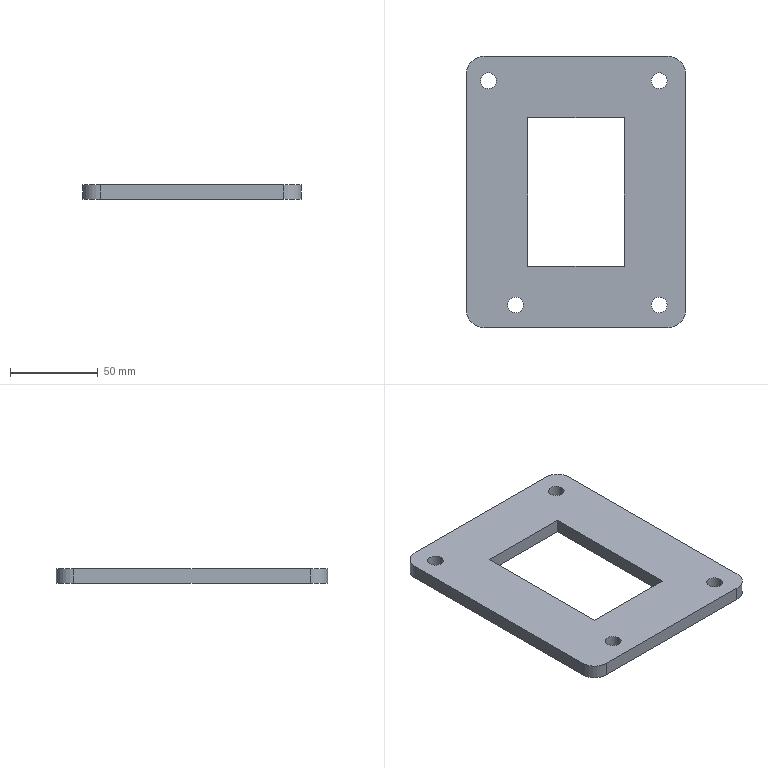Part | SolidWorks | features FlatPattern 1, SMBaseFlange 1, SheetMetal 1 | 1 solid | 22 faces | box 125 x 155 x 8 mm | volume 114878 mm3 | cylinder 12 | plane 10 | commonest cylinder face diameters 9 x8 20 x4
STEP:
#1=CARTESIAN_POINT('',(-51.5,13.,8.));
#2=VERTEX_POINT('',#1);
#3=CARTESIAN_POINT('',(-42.5,13.,8.));
#4=VERTEX_POINT('',#3);
#5=CARTESIAN_POINT('',(-47.,13.,8.));
#6=DIRECTION('',(0.,0.,1.));
#7=DIRECTION('',(1.,0.,0.));
#8=AXIS2_PLACEMENT_3D('',#5,#6,#7);
#9=CIRCLE('',#8,4.5);
#10=EDGE_CURVE('',#2,#4,#9,.T.);
#11=ORIENTED_EDGE('',*,*,#10,.T.);
#12=CARTESIAN_POINT('',(-42.5,13.,0.));
#13=VERTEX_POINT('',#12);
#14=CARTESIAN_POINT('',(-42.5,13.,8.));
#15=DIRECTION('',(0.,0.,-1.));
#16=VECTOR('',#15,1000.);
#17=LINE('',#14,#16);
#18=EDGE_CURVE('',#4,#13,#17,.T.);
#19=ORIENTED_EDGE('',*,*,#18,.T.);
#20=CARTESIAN_POINT('',(-51.5,13.,0.));
#21=VERTEX_POINT('',#20);
#22=CARTESIAN_POINT('',(-47.,13.,0.));
#23=DIRECTION('',(0.,0.,1.));
#24=DIRECTION('',(1.,0.,0.));
#25=AXIS2_PLACEMENT_3D('',#22,#23,#24);
#26=CIRCLE('',#25,4.5);
#27=EDGE_CURVE('',#21,#13,#26,.T.);
#28=ORIENTED_EDGE('',*,*,#27,.F.);
#29=CARTESIAN_POINT('',(-51.5,13.,8.));
#30=DIRECTION('',(0.,0.,-1.));
#31=VECTOR('',#30,1000.);
#32=LINE('',#29,#31);
#33=EDGE_CURVE('',#2,#21,#32,.T.);
#34=ORIENTED_EDGE('',*,*,#33,.F.);
#35=EDGE_LOOP('',(#11,#19,#28,#34));
#36=FACE_OUTER_BOUND('',#35,.T.);
#37=CARTESIAN_POINT('',(-47.,13.,8.));
#38=DIRECTION('',(0.,0.,-1.));
#39=DIRECTION('',(-1.,0.,0.));
#40=AXIS2_PLACEMENT_3D('',#37,#38,#39);
#41=CYLINDRICAL_SURFACE('',#40,4.5);
#42=ADVANCED_FACE('',(#36),#41,.F.);
#43=CARTESIAN_POINT('',(30.5,13.,8.));
#44=VERTEX_POINT('',#43);
#45=CARTESIAN_POINT('',(39.5,13.,8.));
#46=VERTEX_POINT('',#45);
#47=CARTESIAN_POINT('',(35.,13.,8.));
#48=DIRECTION('',(0.,0.,1.));
#49=DIRECTION('',(1.,0.,0.));
#50=AXIS2_PLACEMENT_3D('',#47,#48,#49);
#51=CIRCLE('',#50,4.5);
#52=EDGE_CURVE('',#44,#46,#51,.T.);
#53=ORIENTED_EDGE('',*,*,#52,.T.);
#54=CARTESIAN_POINT('',(39.5,13.,0.));
#55=VERTEX_POINT('',#54);
#56=CARTESIAN_POINT('',(39.5,13.,8.));
#57=DIRECTION('',(0.,0.,-1.));
#58=VECTOR('',#57,1000.);
#59=LINE('',#56,#58);
#60=EDGE_CURVE('',#46,#55,#59,.T.);
#61=ORIENTED_EDGE('',*,*,#60,.T.);
#62=CARTESIAN_POINT('',(30.5,13.,0.));
#63=VERTEX_POINT('',#62);
#64=CARTESIAN_POINT('',(35.,13.,0.));
#65=DIRECTION('',(0.,0.,1.));
#66=DIRECTION('',(1.,0.,0.));
#67=AXIS2_PLACEMENT_3D('',#64,#65,#66);
#68=CIRCLE('',#67,4.5);
#69=EDGE_CURVE('',#63,#55,#68,.T.);
#70=ORIENTED_EDGE('',*,*,#69,.F.);
#71=CARTESIAN_POINT('',(30.5,13.,8.));
#72=DIRECTION('',(0.,0.,-1.));
#73=VECTOR('',#72,1000.);
#74=LINE('',#71,#73);
#75=EDGE_CURVE('',#44,#63,#74,.T.);
#76=ORIENTED_EDGE('',*,*,#75,.F.);
#77=EDGE_LOOP('',(#53,#61,#70,#76));
#78=FACE_OUTER_BOUND('',#77,.T.);
#79=CARTESIAN_POINT('',(35.,13.,8.));
#80=DIRECTION('',(0.,0.,-1.));
#81=DIRECTION('',(-1.,0.,0.));
#82=AXIS2_PLACEMENT_3D('',#79,#80,#81);
#83=CYLINDRICAL_SURFACE('',#82,4.5);
#84=ADVANCED_FACE('',(#78),#83,.F.);
#85=CARTESIAN_POINT('',(30.5,141.,8.));
#86=VERTEX_POINT('',#85);
#87=CARTESIAN_POINT('',(39.5,141.,8.));
#88=VERTEX_POINT('',#87);
#89=CARTESIAN_POINT('',(35.,141.,8.));
#90=DIRECTION('',(0.,0.,1.));
#91=DIRECTION('',(1.,0.,0.));
#92=AXIS2_PLACEMENT_3D('',#89,#90,#91);
#93=CIRCLE('',#92,4.5);
#94=EDGE_CURVE('',#86,#88,#93,.T.);
#95=ORIENTED_EDGE('',*,*,#94,.T.);
#96=CARTESIAN_POINT('',(39.5,141.,0.));
#97=VERTEX_POINT('',#96);
#98=CARTESIAN_POINT('',(39.5,141.,8.));
#99=DIRECTION('',(0.,0.,-1.));
#100=VECTOR('',#99,1000.);
#101=LINE('',#98,#100);
#102=EDGE_CURVE('',#88,#97,#101,.T.);
#103=ORIENTED_EDGE('',*,*,#102,.T.);
#104=CARTESIAN_POINT('',(30.5,141.,0.));
#105=VERTEX_POINT('',#104);
#106=CARTESIAN_POINT('',(35.,141.,0.));
#107=DIRECTION('',(0.,0.,1.));
#108=DIRECTION('',(1.,0.,0.));
#109=AXIS2_PLACEMENT_3D('',#106,#107,#108);
#110=CIRCLE('',#109,4.5);
#111=EDGE_CURVE('',#105,#97,#110,.T.);
#112=ORIENTED_EDGE('',*,*,#111,.F.);
#113=CARTESIAN_POINT('',(30.5,141.,8.));
#114=DIRECTION('',(0.,0.,-1.));
#115=VECTOR('',#114,1000.);
#116=LINE('',#113,#115);
#117=EDGE_CURVE('',#86,#105,#116,.T.);
#118=ORIENTED_EDGE('',*,*,#117,.F.);
#119=EDGE_LOOP('',(#95,#103,#112,#118));
#120=FACE_OUTER_BOUND('',#119,.T.);
#121=CARTESIAN_POINT('',(35.,141.,8.));
#122=DIRECTION('',(0.,0.,-1.));
#123=DIRECTION('',(-1.,0.,0.));
#124=AXIS2_PLACEMENT_3D('',#121,#122,#123);
#125=CYLINDRICAL_SURFACE('',#124,4.5);
#126=ADVANCED_FACE('',(#120),#125,.F.);
#127=CARTESIAN_POINT('',(-67.,141.,8.));
#128=VERTEX_POINT('',#127);
#129=CARTESIAN_POINT('',(-58.,141.,8.));
#130=VERTEX_POINT('',#129);
#131=CARTESIAN_POINT('',(-62.5,141.,8.));
#132=DIRECTION('',(0.,0.,1.));
#133=DIRECTION('',(1.,0.,0.));
#134=AXIS2_PLACEMENT_3D('',#131,#132,#133);
#135=CIRCLE('',#134,4.5);
#136=EDGE_CURVE('',#128,#130,#135,.T.);
#137=ORIENTED_EDGE('',*,*,#136,.T.);
#138=CARTESIAN_POINT('',(-58.,141.,0.));
#139=VERTEX_POINT('',#138);
#140=CARTESIAN_POINT('',(-58.,141.,8.));
#141=DIRECTION('',(0.,0.,-1.));
#142=VECTOR('',#141,1000.);
#143=LINE('',#140,#142);
#144=EDGE_CURVE('',#130,#139,#143,.T.);
#145=ORIENTED_EDGE('',*,*,#144,.T.);
#146=CARTESIAN_POINT('',(-67.,141.,0.));
#147=VERTEX_POINT('',#146);
#148=CARTESIAN_POINT('',(-62.5,141.,0.));
#149=DIRECTION('',(0.,0.,1.));
#150=DIRECTION('',(1.,0.,0.));
#151=AXIS2_PLACEMENT_3D('',#148,#149,#150);
#152=CIRCLE('',#151,4.5);
#153=EDGE_CURVE('',#147,#139,#152,.T.);
#154=ORIENTED_EDGE('',*,*,#153,.F.);
#155=CARTESIAN_POINT('',(-67.,141.,8.));
#156=DIRECTION('',(0.,0.,-1.));
#157=VECTOR('',#156,1000.);
#158=LINE('',#155,#157);
#159=EDGE_CURVE('',#128,#147,#158,.T.);
#160=ORIENTED_EDGE('',*,*,#159,.F.);
#161=EDGE_LOOP('',(#137,#145,#154,#160));
#162=FACE_OUTER_BOUND('',#161,.T.);
#163=CARTESIAN_POINT('',(-62.5,141.,8.));
#164=DIRECTION('',(0.,0.,-1.));
#165=DIRECTION('',(-1.,0.,0.));
#166=AXIS2_PLACEMENT_3D('',#163,#164,#165);
#167=CYLINDRICAL_SURFACE('',#166,4.5);
#168=ADVANCED_FACE('',(#162),#167,.F.);
#169=CARTESIAN_POINT('',(40.,0.,8.));
#170=VERTEX_POINT('',#169);
#171=CARTESIAN_POINT('',(50.,10.,8.));
#172=VERTEX_POINT('',#171);
#173=CARTESIAN_POINT('',(40.,10.,8.));
#174=DIRECTION('',(0.,0.,1.));
#175=DIRECTION('',(-1.,0.,0.));
#176=AXIS2_PLACEMENT_3D('',#173,#174,#175);
#177=CIRCLE('',#176,10.);
#178=EDGE_CURVE('',#170,#172,#177,.T.);
#179=ORIENTED_EDGE('',*,*,#178,.T.);
#180=CARTESIAN_POINT('',(50.,145.,8.));
#181=VERTEX_POINT('',#180);
#182=CARTESIAN_POINT('',(50.,145.,8.));
#183=DIRECTION('',(0.,1.,0.));
#184=VECTOR('',#183,1000.);
#185=LINE('',#182,#184);
#186=EDGE_CURVE('',#172,#181,#185,.T.);
#187=ORIENTED_EDGE('',*,*,#186,.T.);
#188=CARTESIAN_POINT('',(40.,155.,8.));
#189=VERTEX_POINT('',#188);
#190=CARTESIAN_POINT('',(40.,145.,8.));
#191=DIRECTION('',(0.,0.,1.));
#192=DIRECTION('',(-1.,0.,0.));
#193=AXIS2_PLACEMENT_3D('',#190,#191,#192);
#194=CIRCLE('',#193,10.);
#195=EDGE_CURVE('',#181,#189,#194,.T.);
#196=ORIENTED_EDGE('',*,*,#195,.T.);
#197=CARTESIAN_POINT('',(-65.,155.,8.));
#198=VERTEX_POINT('',#197);
#199=CARTESIAN_POINT('',(40.,155.,8.));
#200=DIRECTION('',(-1.,0.,0.));
#201=VECTOR('',#200,1000.);
#202=LINE('',#199,#201);
#203=EDGE_CURVE('',#189,#198,#202,.T.);
#204=ORIENTED_EDGE('',*,*,#203,.T.);
#205=CARTESIAN_POINT('',(-75.,145.,8.));
#206=VERTEX_POINT('',#205);
#207=CARTESIAN_POINT('',(-65.,145.,8.));
#208=DIRECTION('',(0.,0.,1.));
#209=DIRECTION('',(1.,0.,0.));
#210=AXIS2_PLACEMENT_3D('',#207,#208,#209);
#211=CIRCLE('',#210,10.);
#212=EDGE_CURVE('',#198,#206,#211,.T.);
#213=ORIENTED_EDGE('',*,*,#212,.T.);
#214=CARTESIAN_POINT('',(-75.,10.,8.));
#215=VERTEX_POINT('',#214);
#216=CARTESIAN_POINT('',(-75.,145.,8.));
#217=DIRECTION('',(0.,-1.,0.));
#218=VECTOR('',#217,1000.);
#219=LINE('',#216,#218);
#220=EDGE_CURVE('',#206,#215,#219,.T.);
#221=ORIENTED_EDGE('',*,*,#220,.T.);
#222=CARTESIAN_POINT('',(-65.,0.,8.));
#223=VERTEX_POINT('',#222);
#224=CARTESIAN_POINT('',(-65.,10.,8.));
#225=DIRECTION('',(0.,0.,1.));
#226=DIRECTION('',(-1.,0.,0.));
#227=AXIS2_PLACEMENT_3D('',#224,#225,#226);
#228=CIRCLE('',#227,10.);
#229=EDGE_CURVE('',#215,#223,#228,.T.);
#230=ORIENTED_EDGE('',*,*,#229,.T.);
#231=CARTESIAN_POINT('',(40.,0.,8.));
#232=DIRECTION('',(1.,0.,0.));
#233=VECTOR('',#232,1000.);
#234=LINE('',#231,#233);
#235=EDGE_CURVE('',#223,#170,#234,.T.);
#236=ORIENTED_EDGE('',*,*,#235,.T.);
#237=EDGE_LOOP('',(#179,#187,#196,#204,#213,#221,#230,#236));
#238=FACE_OUTER_BOUND('',#237,.T.);
#239=CARTESIAN_POINT('',(15.,35.,8.));
#240=VERTEX_POINT('',#239);
#241=CARTESIAN_POINT('',(15.,120.,8.));
#242=VERTEX_POINT('',#241);
#243=CARTESIAN_POINT('',(15.,120.,8.));
#244=DIRECTION('',(0.,1.,0.));
#245=VECTOR('',#244,1000.);
#246=LINE('',#243,#245);
#247=EDGE_CURVE('',#240,#242,#246,.T.);
#248=ORIENTED_EDGE('',*,*,#247,.F.);
#249=CARTESIAN_POINT('',(-40.,35.,8.));
#250=VERTEX_POINT('',#249);
#251=CARTESIAN_POINT('',(15.,35.,8.));
#252=DIRECTION('',(1.,0.,0.));
#253=VECTOR('',#252,1000.);
#254=LINE('',#251,#253);
#255=EDGE_CURVE('',#250,#240,#254,.T.);
#256=ORIENTED_EDGE('',*,*,#255,.F.);
#257=CARTESIAN_POINT('',(-40.,120.,8.));
#258=VERTEX_POINT('',#257);
#259=CARTESIAN_POINT('',(-40.,120.,8.));
#260=DIRECTION('',(0.,-1.,0.));
#261=VECTOR('',#260,1000.);
#262=LINE('',#259,#261);
#263=EDGE_CURVE('',#258,#250,#262,.T.);
#264=ORIENTED_EDGE('',*,*,#263,.F.);
#265=CARTESIAN_POINT('',(15.,120.,8.));
#266=DIRECTION('',(-1.,0.,0.));
#267=VECTOR('',#266,1000.);
#268=LINE('',#265,#267);
#269=EDGE_CURVE('',#242,#258,#268,.T.);
#270=ORIENTED_EDGE('',*,*,#269,.F.);
#271=EDGE_LOOP('',(#248,#256,#264,#270));
#272=FACE_BOUND('',#271,.T.);
#273=ORIENTED_EDGE('',*,*,#136,.F.);
#274=CARTESIAN_POINT('',(-62.5,141.,8.));
#275=DIRECTION('',(0.,0.,1.));
#276=DIRECTION('',(1.,0.,0.));
#277=AXIS2_PLACEMENT_3D('',#274,#275,#276);
#278=CIRCLE('',#277,4.5);
#279=EDGE_CURVE('',#130,#128,#278,.T.);
#280=ORIENTED_EDGE('',*,*,#279,.F.);
#281=EDGE_LOOP('',(#273,#280));
#282=FACE_BOUND('',#281,.T.);
#283=ORIENTED_EDGE('',*,*,#94,.F.);
#284=CARTESIAN_POINT('',(35.,141.,8.));
#285=DIRECTION('',(0.,0.,1.));
#286=DIRECTION('',(1.,0.,0.));
#287=AXIS2_PLACEMENT_3D('',#284,#285,#286);
#288=CIRCLE('',#287,4.5);
#289=EDGE_CURVE('',#88,#86,#288,.T.);
#290=ORIENTED_EDGE('',*,*,#289,.F.);
#291=EDGE_LOOP('',(#283,#290));
#292=FACE_BOUND('',#291,.T.);
#293=ORIENTED_EDGE('',*,*,#52,.F.);
#294=CARTESIAN_POINT('',(35.,13.,8.));
#295=DIRECTION('',(0.,0.,1.));
#296=DIRECTION('',(1.,0.,0.));
#297=AXIS2_PLACEMENT_3D('',#294,#295,#296);
#298=CIRCLE('',#297,4.5);
#299=EDGE_CURVE('',#46,#44,#298,.T.);
#300=ORIENTED_EDGE('',*,*,#299,.F.);
#301=EDGE_LOOP('',(#293,#300));
#302=FACE_BOUND('',#301,.T.);
#303=ORIENTED_EDGE('',*,*,#10,.F.);
#304=CARTESIAN_POINT('',(-47.,13.,8.));
#305=DIRECTION('',(0.,0.,1.));
#306=DIRECTION('',(1.,0.,0.));
#307=AXIS2_PLACEMENT_3D('',#304,#305,#306);
#308=CIRCLE('',#307,4.5);
#309=EDGE_CURVE('',#4,#2,#308,.T.);
#310=ORIENTED_EDGE('',*,*,#309,.F.);
#311=EDGE_LOOP('',(#303,#310));
#312=FACE_BOUND('',#311,.T.);
#313=CARTESIAN_POINT('',(40.,10.,8.));
#314=DIRECTION('',(0.,0.,-1.));
#315=DIRECTION('',(-1.,0.,0.));
#316=AXIS2_PLACEMENT_3D('',#313,#314,#315);
#317=PLANE('',#316);
#318=ADVANCED_FACE('',(#238,#272,#282,#292,#302,#312),#317,.F.);
#319=ORIENTED_EDGE('',*,*,#69,.T.);
#320=CARTESIAN_POINT('',(35.,13.,0.));
#321=DIRECTION('',(0.,0.,1.));
#322=DIRECTION('',(1.,0.,0.));
#323=AXIS2_PLACEMENT_3D('',#320,#321,#322);
#324=CIRCLE('',#323,4.5);
#325=EDGE_CURVE('',#55,#63,#324,.T.);
#326=ORIENTED_EDGE('',*,*,#325,.T.);
#327=EDGE_LOOP('',(#319,#326));
#328=FACE_BOUND('',#327,.T.);
#329=ORIENTED_EDGE('',*,*,#153,.T.);
#330=CARTESIAN_POINT('',(-62.5,141.,0.));
#331=DIRECTION('',(0.,0.,1.));
#332=DIRECTION('',(1.,0.,0.));
#333=AXIS2_PLACEMENT_3D('',#330,#331,#332);
#334=CIRCLE('',#333,4.5);
#335=EDGE_CURVE('',#139,#147,#334,.T.);
#336=ORIENTED_EDGE('',*,*,#335,.T.);
#337=EDGE_LOOP('',(#329,#336));
#338=FACE_BOUND('',#337,.T.);
#339=CARTESIAN_POINT('',(40.,0.,0.));
#340=VERTEX_POINT('',#339);
#341=CARTESIAN_POINT('',(50.,10.,0.));
#342=VERTEX_POINT('',#341);
#343=CARTESIAN_POINT('',(40.,10.,0.));
#344=DIRECTION('',(0.,0.,1.));
#345=DIRECTION('',(-1.,0.,0.));
#346=AXIS2_PLACEMENT_3D('',#343,#344,#345);
#347=CIRCLE('',#346,10.);
#348=EDGE_CURVE('',#340,#342,#347,.T.);
#349=ORIENTED_EDGE('',*,*,#348,.F.);
#350=CARTESIAN_POINT('',(-65.,0.,0.));
#351=VERTEX_POINT('',#350);
#352=CARTESIAN_POINT('',(40.,0.,0.));
#353=DIRECTION('',(1.,0.,0.));
#354=VECTOR('',#353,1000.);
#355=LINE('',#352,#354);
#356=EDGE_CURVE('',#351,#340,#355,.T.);
#357=ORIENTED_EDGE('',*,*,#356,.F.);
#358=CARTESIAN_POINT('',(-75.,10.,0.));
#359=VERTEX_POINT('',#358);
#360=CARTESIAN_POINT('',(-65.,10.,0.));
#361=DIRECTION('',(0.,0.,1.));
#362=DIRECTION('',(-1.,0.,0.));
#363=AXIS2_PLACEMENT_3D('',#360,#361,#362);
#364=CIRCLE('',#363,10.);
#365=EDGE_CURVE('',#359,#351,#364,.T.);
#366=ORIENTED_EDGE('',*,*,#365,.F.);
#367=CARTESIAN_POINT('',(-75.,145.,0.));
#368=VERTEX_POINT('',#367);
#369=CARTESIAN_POINT('',(-75.,145.,0.));
#370=DIRECTION('',(0.,-1.,0.));
#371=VECTOR('',#370,1000.);
#372=LINE('',#369,#371);
#373=EDGE_CURVE('',#368,#359,#372,.T.);
#374=ORIENTED_EDGE('',*,*,#373,.F.);
#375=CARTESIAN_POINT('',(-65.,155.,0.));
#376=VERTEX_POINT('',#375);
#377=CARTESIAN_POINT('',(-65.,145.,0.));
#378=DIRECTION('',(0.,0.,1.));
#379=DIRECTION('',(1.,0.,0.));
#380=AXIS2_PLACEMENT_3D('',#377,#378,#379);
#381=CIRCLE('',#380,10.);
#382=EDGE_CURVE('',#376,#368,#381,.T.);
#383=ORIENTED_EDGE('',*,*,#382,.F.);
#384=CARTESIAN_POINT('',(40.,155.,0.));
#385=VERTEX_POINT('',#384);
#386=CARTESIAN_POINT('',(40.,155.,0.));
#387=DIRECTION('',(-1.,0.,0.));
#388=VECTOR('',#387,1000.);
#389=LINE('',#386,#388);
#390=EDGE_CURVE('',#385,#376,#389,.T.);
#391=ORIENTED_EDGE('',*,*,#390,.F.);
#392=CARTESIAN_POINT('',(50.,145.,0.));
#393=VERTEX_POINT('',#392);
#394=CARTESIAN_POINT('',(40.,145.,0.));
#395=DIRECTION('',(0.,0.,1.));
#396=DIRECTION('',(-1.,0.,0.));
#397=AXIS2_PLACEMENT_3D('',#394,#395,#396);
#398=CIRCLE('',#397,10.);
#399=EDGE_CURVE('',#393,#385,#398,.T.);
#400=ORIENTED_EDGE('',*,*,#399,.F.);
#401=CARTESIAN_POINT('',(50.,145.,0.));
#402=DIRECTION('',(0.,1.,0.));
#403=VECTOR('',#402,1000.);
#404=LINE('',#401,#403);
#405=EDGE_CURVE('',#342,#393,#404,.T.);
#406=ORIENTED_EDGE('',*,*,#405,.F.);
#407=EDGE_LOOP('',(#349,#357,#366,#374,#383,#391,#400,#406));
#408=FACE_OUTER_BOUND('',#407,.T.);
#409=CARTESIAN_POINT('',(-40.,35.,0.));
#410=VERTEX_POINT('',#409);
#411=CARTESIAN_POINT('',(15.,35.,0.));
#412=VERTEX_POINT('',#411);
#413=CARTESIAN_POINT('',(15.,35.,0.));
#414=DIRECTION('',(1.,0.,0.));
#415=VECTOR('',#414,1000.);
#416=LINE('',#413,#415);
#417=EDGE_CURVE('',#410,#412,#416,.T.);
#418=ORIENTED_EDGE('',*,*,#417,.T.);
#419=CARTESIAN_POINT('',(15.,120.,0.));
#420=VERTEX_POINT('',#419);
#421=CARTESIAN_POINT('',(15.,120.,0.));
#422=DIRECTION('',(0.,1.,0.));
#423=VECTOR('',#422,1000.);
#424=LINE('',#421,#423);
#425=EDGE_CURVE('',#412,#420,#424,.T.);
#426=ORIENTED_EDGE('',*,*,#425,.T.);
#427=CARTESIAN_POINT('',(-40.,120.,0.));
#428=VERTEX_POINT('',#427);
#429=CARTESIAN_POINT('',(15.,120.,0.));
#430=DIRECTION('',(-1.,0.,0.));
#431=VECTOR('',#430,1000.);
#432=LINE('',#429,#431);
#433=EDGE_CURVE('',#420,#428,#432,.T.);
#434=ORIENTED_EDGE('',*,*,#433,.T.);
#435=CARTESIAN_POINT('',(-40.,120.,0.));
#436=DIRECTION('',(0.,-1.,0.));
#437=VECTOR('',#436,1000.);
#438=LINE('',#435,#437);
#439=EDGE_CURVE('',#428,#410,#438,.T.);
#440=ORIENTED_EDGE('',*,*,#439,.T.);
#441=EDGE_LOOP('',(#418,#426,#434,#440));
#442=FACE_BOUND('',#441,.T.);
#443=ORIENTED_EDGE('',*,*,#111,.T.);
#444=CARTESIAN_POINT('',(35.,141.,0.));
#445=DIRECTION('',(0.,0.,1.));
#446=DIRECTION('',(1.,0.,0.));
#447=AXIS2_PLACEMENT_3D('',#444,#445,#446);
#448=CIRCLE('',#447,4.5);
#449=EDGE_CURVE('',#97,#105,#448,.T.);
#450=ORIENTED_EDGE('',*,*,#449,.T.);
#451=EDGE_LOOP('',(#443,#450));
#452=FACE_BOUND('',#451,.T.);
#453=ORIENTED_EDGE('',*,*,#27,.T.);
#454=CARTESIAN_POINT('',(-47.,13.,0.));
#455=DIRECTION('',(0.,0.,1.));
#456=DIRECTION('',(1.,0.,0.));
#457=AXIS2_PLACEMENT_3D('',#454,#455,#456);
#458=CIRCLE('',#457,4.5);
#459=EDGE_CURVE('',#13,#21,#458,.T.);
#460=ORIENTED_EDGE('',*,*,#459,.T.);
#461=EDGE_LOOP('',(#453,#460));
#462=FACE_BOUND('',#461,.T.);
#463=CARTESIAN_POINT('',(40.,10.,0.));
#464=DIRECTION('',(0.,0.,-1.));
#465=DIRECTION('',(-1.,0.,0.));
#466=AXIS2_PLACEMENT_3D('',#463,#464,#465);
#467=PLANE('',#466);
#468=ADVANCED_FACE('',(#328,#338,#408,#442,#452,#462),#467,.T.);
#469=ORIENTED_EDGE('',*,*,#348,.T.);
#470=CARTESIAN_POINT('',(50.,10.,8.));
#471=DIRECTION('',(0.,0.,-1.));
#472=VECTOR('',#471,1000.);
#473=LINE('',#470,#472);
#474=EDGE_CURVE('',#172,#342,#473,.T.);
#475=ORIENTED_EDGE('',*,*,#474,.F.);
#476=ORIENTED_EDGE('',*,*,#178,.F.);
#477=CARTESIAN_POINT('',(40.,0.,8.));
#478=DIRECTION('',(0.,0.,-1.));
#479=VECTOR('',#478,1000.);
#480=LINE('',#477,#479);
#481=EDGE_CURVE('',#170,#340,#480,.T.);
#482=ORIENTED_EDGE('',*,*,#481,.T.);
#483=EDGE_LOOP('',(#469,#475,#476,#482));
#484=FACE_OUTER_BOUND('',#483,.T.);
#485=CARTESIAN_POINT('',(40.,10.,8.));
#486=DIRECTION('',(0.,0.,-1.));
#487=DIRECTION('',(-1.,0.,0.));
#488=AXIS2_PLACEMENT_3D('',#485,#486,#487);
#489=CYLINDRICAL_SURFACE('',#488,10.);
#490=ADVANCED_FACE('',(#484),#489,.T.);
#491=ORIENTED_EDGE('',*,*,#405,.T.);
#492=CARTESIAN_POINT('',(50.,145.,8.));
#493=DIRECTION('',(0.,0.,-1.));
#494=VECTOR('',#493,1000.);
#495=LINE('',#492,#494);
#496=EDGE_CURVE('',#181,#393,#495,.T.);
#497=ORIENTED_EDGE('',*,*,#496,.F.);
#498=ORIENTED_EDGE('',*,*,#186,.F.);
#499=ORIENTED_EDGE('',*,*,#474,.T.);
#500=EDGE_LOOP('',(#491,#497,#498,#499));
#501=FACE_OUTER_BOUND('',#500,.T.);
#502=CARTESIAN_POINT('',(50.,145.,8.));
#503=DIRECTION('',(-1.,0.,0.));
#504=DIRECTION('',(0.,-1.,0.));
#505=AXIS2_PLACEMENT_3D('',#502,#503,#504);
#506=PLANE('',#505);
#507=ADVANCED_FACE('',(#501),#506,.F.);
#508=ORIENTED_EDGE('',*,*,#399,.T.);
#509=CARTESIAN_POINT('',(40.,155.,8.));
#510=DIRECTION('',(0.,0.,-1.));
#511=VECTOR('',#510,1000.);
#512=LINE('',#509,#511);
#513=EDGE_CURVE('',#189,#385,#512,.T.);
#514=ORIENTED_EDGE('',*,*,#513,.F.);
#515=ORIENTED_EDGE('',*,*,#195,.F.);
#516=ORIENTED_EDGE('',*,*,#496,.T.);
#517=EDGE_LOOP('',(#508,#514,#515,#516));
#518=FACE_OUTER_BOUND('',#517,.T.);
#519=CARTESIAN_POINT('',(40.,145.,8.));
#520=DIRECTION('',(0.,0.,-1.));
#521=DIRECTION('',(-1.,0.,0.));
#522=AXIS2_PLACEMENT_3D('',#519,#520,#521);
#523=CYLINDRICAL_SURFACE('',#522,10.);
#524=ADVANCED_FACE('',(#518),#523,.T.);
#525=ORIENTED_EDGE('',*,*,#390,.T.);
#526=CARTESIAN_POINT('',(-65.,155.,8.));
#527=DIRECTION('',(0.,0.,-1.));
#528=VECTOR('',#527,1000.);
#529=LINE('',#526,#528);
#530=EDGE_CURVE('',#198,#376,#529,.T.);
#531=ORIENTED_EDGE('',*,*,#530,.F.);
#532=ORIENTED_EDGE('',*,*,#203,.F.);
#533=ORIENTED_EDGE('',*,*,#513,.T.);
#534=EDGE_LOOP('',(#525,#531,#532,#533));
#535=FACE_OUTER_BOUND('',#534,.T.);
#536=CARTESIAN_POINT('',(40.,155.,8.));
#537=DIRECTION('',(0.,-1.,0.));
#538=DIRECTION('',(0.,0.,-1.));
#539=AXIS2_PLACEMENT_3D('',#536,#537,#538);
#540=PLANE('',#539);
#541=ADVANCED_FACE('',(#535),#540,.F.);
#542=ORIENTED_EDGE('',*,*,#382,.T.);
#543=CARTESIAN_POINT('',(-75.,145.,8.));
#544=DIRECTION('',(0.,0.,-1.));
#545=VECTOR('',#544,1000.);
#546=LINE('',#543,#545);
#547=EDGE_CURVE('',#206,#368,#546,.T.);
#548=ORIENTED_EDGE('',*,*,#547,.F.);
#549=ORIENTED_EDGE('',*,*,#212,.F.);
#550=ORIENTED_EDGE('',*,*,#530,.T.);
#551=EDGE_LOOP('',(#542,#548,#549,#550));
#552=FACE_OUTER_BOUND('',#551,.T.);
#553=CARTESIAN_POINT('',(-65.,145.,8.));
#554=DIRECTION('',(0.,0.,-1.));
#555=DIRECTION('',(-1.,0.,0.));
#556=AXIS2_PLACEMENT_3D('',#553,#554,#555);
#557=CYLINDRICAL_SURFACE('',#556,10.);
#558=ADVANCED_FACE('',(#552),#557,.T.);
#559=ORIENTED_EDGE('',*,*,#373,.T.);
#560=CARTESIAN_POINT('',(-75.,10.,8.));
#561=DIRECTION('',(0.,0.,-1.));
#562=VECTOR('',#561,1000.);
#563=LINE('',#560,#562);
#564=EDGE_CURVE('',#215,#359,#563,.T.);
#565=ORIENTED_EDGE('',*,*,#564,.F.);
#566=ORIENTED_EDGE('',*,*,#220,.F.);
#567=ORIENTED_EDGE('',*,*,#547,.T.);
#568=EDGE_LOOP('',(#559,#565,#566,#567));
#569=FACE_OUTER_BOUND('',#568,.T.);
#570=CARTESIAN_POINT('',(-75.,145.,8.));
#571=DIRECTION('',(1.,0.,0.));
#572=DIRECTION('',(0.,0.,-1.));
#573=AXIS2_PLACEMENT_3D('',#570,#571,#572);
#574=PLANE('',#573);
#575=ADVANCED_FACE('',(#569),#574,.F.);
#576=ORIENTED_EDGE('',*,*,#365,.T.);
#577=CARTESIAN_POINT('',(-65.,0.,8.));
#578=DIRECTION('',(0.,0.,-1.));
#579=VECTOR('',#578,1000.);
#580=LINE('',#577,#579);
#581=EDGE_CURVE('',#223,#351,#580,.T.);
#582=ORIENTED_EDGE('',*,*,#581,.F.);
#583=ORIENTED_EDGE('',*,*,#229,.F.);
#584=ORIENTED_EDGE('',*,*,#564,.T.);
#585=EDGE_LOOP('',(#576,#582,#583,#584));
#586=FACE_OUTER_BOUND('',#585,.T.);
#587=CARTESIAN_POINT('',(-65.,10.,8.));
#588=DIRECTION('',(0.,0.,-1.));
#589=DIRECTION('',(-1.,0.,0.));
#590=AXIS2_PLACEMENT_3D('',#587,#588,#589);
#591=CYLINDRICAL_SURFACE('',#590,10.);
#592=ADVANCED_FACE('',(#586),#591,.T.);
#593=ORIENTED_EDGE('',*,*,#356,.T.);
#594=ORIENTED_EDGE('',*,*,#481,.F.);
#595=ORIENTED_EDGE('',*,*,#235,.F.);
#596=ORIENTED_EDGE('',*,*,#581,.T.);
#597=EDGE_LOOP('',(#593,#594,#595,#596));
#598=FACE_OUTER_BOUND('',#597,.T.);
#599=CARTESIAN_POINT('',(40.,0.,8.));
#600=DIRECTION('',(0.,1.,0.));
#601=DIRECTION('',(-1.,0.,0.));
#602=AXIS2_PLACEMENT_3D('',#599,#600,#601);
#603=PLANE('',#602);
#604=ADVANCED_FACE('',(#598),#603,.F.);
#605=ORIENTED_EDGE('',*,*,#425,.F.);
#606=CARTESIAN_POINT('',(15.,35.,8.));
#607=DIRECTION('',(0.,0.,-1.));
#608=VECTOR('',#607,1000.);
#609=LINE('',#606,#608);
#610=EDGE_CURVE('',#240,#412,#609,.T.);
#611=ORIENTED_EDGE('',*,*,#610,.F.);
#612=ORIENTED_EDGE('',*,*,#247,.T.);
#613=CARTESIAN_POINT('',(15.,120.,8.));
#614=DIRECTION('',(0.,0.,-1.));
#615=VECTOR('',#614,1000.);
#616=LINE('',#613,#615);
#617=EDGE_CURVE('',#242,#420,#616,.T.);
#618=ORIENTED_EDGE('',*,*,#617,.T.);
#619=EDGE_LOOP('',(#605,#611,#612,#618));
#620=FACE_OUTER_BOUND('',#619,.T.);
#621=CARTESIAN_POINT('',(15.,120.,8.));
#622=DIRECTION('',(-1.,0.,0.));
#623=DIRECTION('',(0.,-1.,0.));
#624=AXIS2_PLACEMENT_3D('',#621,#622,#623);
#625=PLANE('',#624);
#626=ADVANCED_FACE('',(#620),#625,.T.);
#627=ORIENTED_EDGE('',*,*,#433,.F.);
#628=ORIENTED_EDGE('',*,*,#617,.F.);
#629=ORIENTED_EDGE('',*,*,#269,.T.);
#630=CARTESIAN_POINT('',(-40.,120.,8.));
#631=DIRECTION('',(0.,0.,-1.));
#632=VECTOR('',#631,1000.);
#633=LINE('',#630,#632);
#634=EDGE_CURVE('',#258,#428,#633,.T.);
#635=ORIENTED_EDGE('',*,*,#634,.T.);
#636=EDGE_LOOP('',(#627,#628,#629,#635));
#637=FACE_OUTER_BOUND('',#636,.T.);
#638=CARTESIAN_POINT('',(15.,120.,8.));
#639=DIRECTION('',(0.,-1.,0.));
#640=DIRECTION('',(0.,0.,-1.));
#641=AXIS2_PLACEMENT_3D('',#638,#639,#640);
#642=PLANE('',#641);
#643=ADVANCED_FACE('',(#637),#642,.T.);
#644=ORIENTED_EDGE('',*,*,#439,.F.);
#645=ORIENTED_EDGE('',*,*,#634,.F.);
#646=ORIENTED_EDGE('',*,*,#263,.T.);
#647=CARTESIAN_POINT('',(-40.,35.,8.));
#648=DIRECTION('',(0.,0.,-1.));
#649=VECTOR('',#648,1000.);
#650=LINE('',#647,#649);
#651=EDGE_CURVE('',#250,#410,#650,.T.);
#652=ORIENTED_EDGE('',*,*,#651,.T.);
#653=EDGE_LOOP('',(#644,#645,#646,#652));
#654=FACE_OUTER_BOUND('',#653,.T.);
#655=CARTESIAN_POINT('',(-40.,120.,8.));
#656=DIRECTION('',(1.,0.,0.));
#657=DIRECTION('',(0.,1.,0.));
#658=AXIS2_PLACEMENT_3D('',#655,#656,#657);
#659=PLANE('',#658);
#660=ADVANCED_FACE('',(#654),#659,.T.);
#661=ORIENTED_EDGE('',*,*,#417,.F.);
#662=ORIENTED_EDGE('',*,*,#651,.F.);
#663=ORIENTED_EDGE('',*,*,#255,.T.);
#664=ORIENTED_EDGE('',*,*,#610,.T.);
#665=EDGE_LOOP('',(#661,#662,#663,#664));
#666=FACE_OUTER_BOUND('',#665,.T.);
#667=CARTESIAN_POINT('',(15.,35.,8.));
#668=DIRECTION('',(0.,1.,0.));
#669=DIRECTION('',(-1.,0.,0.));
#670=AXIS2_PLACEMENT_3D('',#667,#668,#669);
#671=PLANE('',#670);
#672=ADVANCED_FACE('',(#666),#671,.T.);
#673=ORIENTED_EDGE('',*,*,#144,.F.);
#674=ORIENTED_EDGE('',*,*,#279,.T.);
#675=ORIENTED_EDGE('',*,*,#159,.T.);
#676=ORIENTED_EDGE('',*,*,#335,.F.);
#677=EDGE_LOOP('',(#673,#674,#675,#676));
#678=FACE_OUTER_BOUND('',#677,.T.);
#679=CARTESIAN_POINT('',(-62.5,141.,8.));
#680=DIRECTION('',(0.,0.,-1.));
#681=DIRECTION('',(-1.,0.,0.));
#682=AXIS2_PLACEMENT_3D('',#679,#680,#681);
#683=CYLINDRICAL_SURFACE('',#682,4.5);
#684=ADVANCED_FACE('',(#678),#683,.F.);
#685=ORIENTED_EDGE('',*,*,#102,.F.);
#686=ORIENTED_EDGE('',*,*,#289,.T.);
#687=ORIENTED_EDGE('',*,*,#117,.T.);
#688=ORIENTED_EDGE('',*,*,#449,.F.);
#689=EDGE_LOOP('',(#685,#686,#687,#688));
#690=FACE_OUTER_BOUND('',#689,.T.);
#691=CARTESIAN_POINT('',(35.,141.,8.));
#692=DIRECTION('',(0.,0.,-1.));
#693=DIRECTION('',(-1.,0.,0.));
#694=AXIS2_PLACEMENT_3D('',#691,#692,#693);
#695=CYLINDRICAL_SURFACE('',#694,4.5);
#696=ADVANCED_FACE('',(#690),#695,.F.);
#697=ORIENTED_EDGE('',*,*,#60,.F.);
#698=ORIENTED_EDGE('',*,*,#299,.T.);
#699=ORIENTED_EDGE('',*,*,#75,.T.);
#700=ORIENTED_EDGE('',*,*,#325,.F.);
#701=EDGE_LOOP('',(#697,#698,#699,#700));
#702=FACE_OUTER_BOUND('',#701,.T.);
#703=CARTESIAN_POINT('',(35.,13.,8.));
#704=DIRECTION('',(0.,0.,-1.));
#705=DIRECTION('',(-1.,0.,0.));
#706=AXIS2_PLACEMENT_3D('',#703,#704,#705);
#707=CYLINDRICAL_SURFACE('',#706,4.5);
#708=ADVANCED_FACE('',(#702),#707,.F.);
#709=ORIENTED_EDGE('',*,*,#18,.F.);
#710=ORIENTED_EDGE('',*,*,#309,.T.);
#711=ORIENTED_EDGE('',*,*,#33,.T.);
#712=ORIENTED_EDGE('',*,*,#459,.F.);
#713=EDGE_LOOP('',(#709,#710,#711,#712));
#714=FACE_OUTER_BOUND('',#713,.T.);
#715=CARTESIAN_POINT('',(-47.,13.,8.));
#716=DIRECTION('',(0.,0.,-1.));
#717=DIRECTION('',(-1.,0.,0.));
#718=AXIS2_PLACEMENT_3D('',#715,#716,#717);
#719=CYLINDRICAL_SURFACE('',#718,4.5);
#720=ADVANCED_FACE('',(#714),#719,.F.);
#721=CLOSED_SHELL('',(#42,#84,#126,#168,#318,#468,#490,#507,#524,#541,#558,#575,#592,#604,#626,#643,#660,#672,#684,#696,#708,#720));
#722=MANIFOLD_SOLID_BREP('',#721);
#723=CARTESIAN_POINT('',(0.,0.,0.));
#724=DIRECTION('',(0.,0.,1.));
#725=DIRECTION('',(1.,0.,0.));
#726=AXIS2_PLACEMENT_3D('',#723,#724,#725);
#727=(LENGTH_UNIT()NAMED_UNIT(*)SI_UNIT(.MILLI.,.METRE.));
#728=UNCERTAINTY_MEASURE_WITH_UNIT(LENGTH_MEASURE(0.00001),#727,'','');
#729=(NAMED_UNIT(*)PLANE_ANGLE_UNIT()SI_UNIT($,.RADIAN.));
#730=(NAMED_UNIT(*)SI_UNIT($,.STERADIAN.)SOLID_ANGLE_UNIT());
#731=(GEOMETRIC_REPRESENTATION_CONTEXT(3)GLOBAL_UNCERTAINTY_ASSIGNED_CONTEXT((#728))GLOBAL_UNIT_ASSIGNED_CONTEXT((#727,#729,#730))REPRESENTATION_CONTEXT('',''));
#732=ADVANCED_BREP_SHAPE_REPRESENTATION('',(#722,#726),#731);